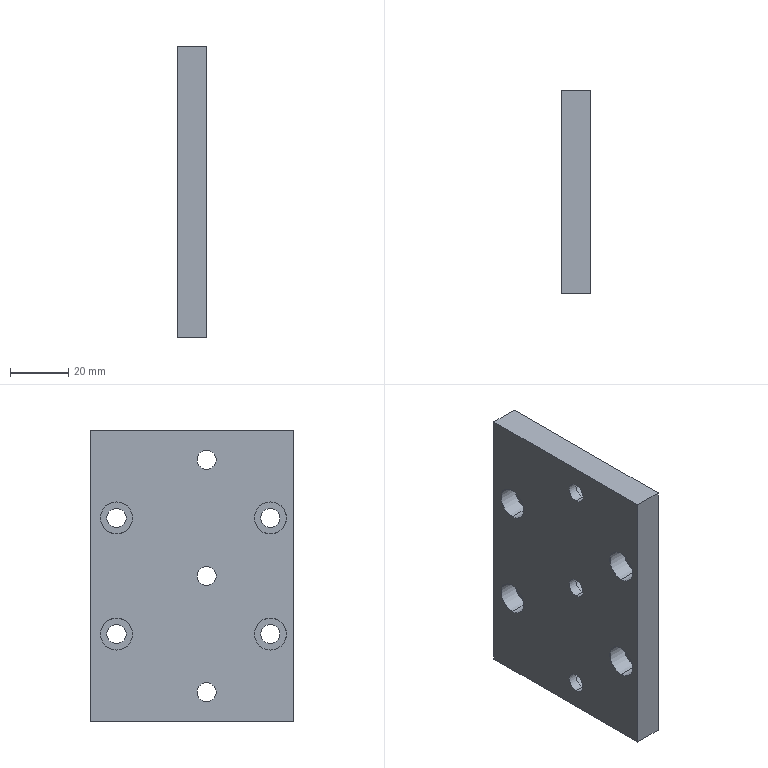Part | SolidWorks | features HoleWzd 3, Extrusion 1 | 1 solid | 57 faces | box 10 x 70 x 100 mm | volume 64355 mm3 | cylinder 32 | plane 13 | cone 12 | commonest cylinder face diameters 6.6 x14 11 x14 4.2 x4